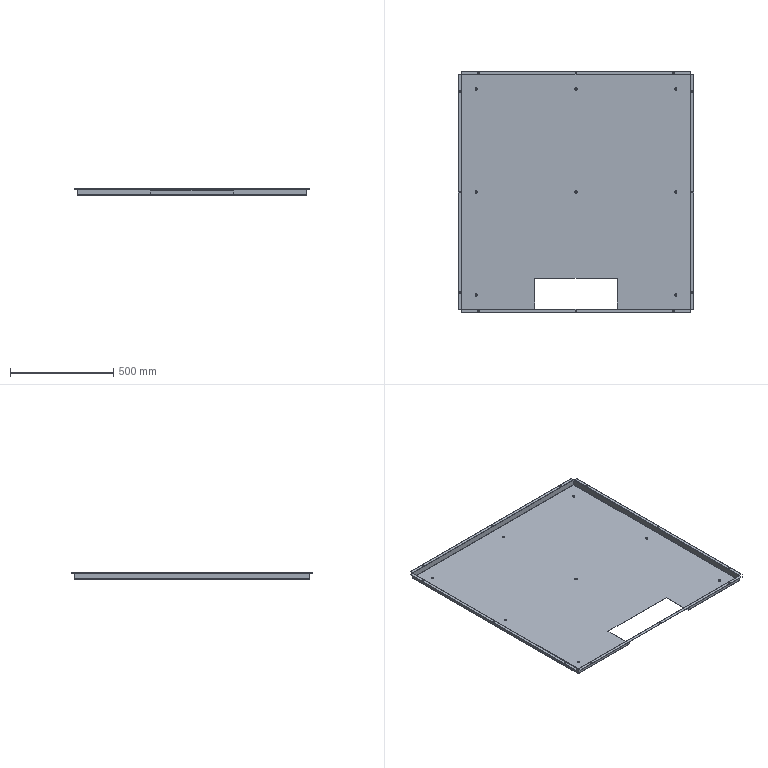Part | 1 solid | 150 faces | box 1140 x 1170 x 30 mm | volume 1390980 mm3 | plane 78 | cylinder 64 | spline 8 | commonest cylinder face diameters 7 x30 11 x16 0.4 x9 2.4 x9